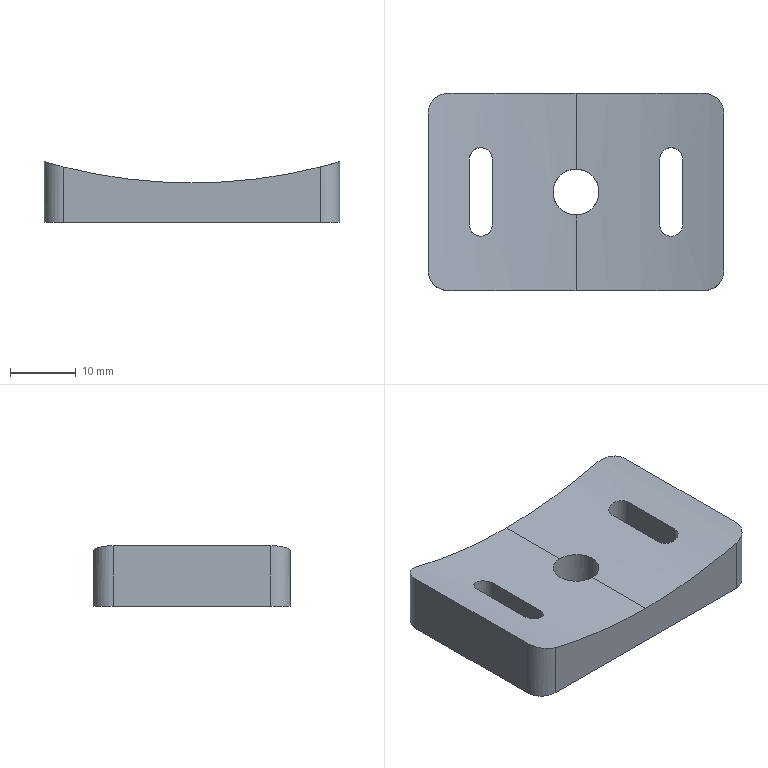Part | SolidWorks | features ICE 2, Extrusion 1, Fillet 1, HoleWzd 1 | 1 solid | 31 faces | box 45 x 30 x 9.229 mm | volume 8297 mm3 | cylinder 16 | plane 15 | commonest cylinder face diameters 6 x8 3.5 x4 7 x2 160 x2
STEP:
#1=CARTESIAN_POINT('',(3.5,15.,-79.923));
#2=VERTEX_POINT('',#1);
#3=CARTESIAN_POINT('',(0.,11.5,-80.));
#4=VERTEX_POINT('',#3);
#5=CARTESIAN_POINT('',(3.5,15.,-79.923));
#6=CARTESIAN_POINT('',(3.5,14.771,-79.923));
#7=CARTESIAN_POINT('',(3.478,14.544,-79.924));
#8=CARTESIAN_POINT('',(3.388,14.093,-79.928));
#9=CARTESIAN_POINT('',(3.321,13.872,-79.931));
#10=CARTESIAN_POINT('',(3.146,13.45,-79.938));
#11=CARTESIAN_POINT('',(3.038,13.247,-79.942));
#12=CARTESIAN_POINT('',(2.782,12.864,-79.952));
#13=CARTESIAN_POINT('',(2.637,12.687,-79.957));
#14=CARTESIAN_POINT('',(2.314,12.364,-79.967));
#15=CARTESIAN_POINT('',(2.134,12.217,-79.972));
#16=CARTESIAN_POINT('',(1.753,11.962,-79.981));
#17=CARTESIAN_POINT('',(1.552,11.855,-79.985));
#18=CARTESIAN_POINT('',(1.129,11.679,-79.992));
#19=CARTESIAN_POINT('',(0.906,11.612,-79.995));
#20=CARTESIAN_POINT('',(0.4583,11.523,-79.999));
#21=CARTESIAN_POINT('',(0.231,11.5,-80.));
#22=CARTESIAN_POINT('',(0.,11.5,-80.));
#23=B_SPLINE_CURVE_WITH_KNOTS('',3,(#5,#6,#7,#8,#9,#10,#11,#12,#13,#14,#15,#16,#17,#18,#19,#20,#21,#22),.UNSPECIFIED.,.F.,.F.,(4,2,2,2,2,2,2,2,4),(0.01094,0.01163,0.01231,0.013,0.01368,0.01436,0.01505,0.01573,0.01642),.UNSPECIFIED.);
#24=EDGE_CURVE('',#2,#4,#23,.T.);
#25=ORIENTED_EDGE('',*,*,#24,.F.);
#26=CARTESIAN_POINT('',(3.5,15.,-86.));
#27=VERTEX_POINT('',#26);
#28=CARTESIAN_POINT('',(3.5,15.,-86.));
#29=DIRECTION('',(0.,0.,-1.));
#30=VECTOR('',#29,1000.);
#31=LINE('',#28,#30);
#32=EDGE_CURVE('',#2,#27,#31,.T.);
#33=ORIENTED_EDGE('',*,*,#32,.T.);
#34=CARTESIAN_POINT('',(-3.5,15.,-86.));
#35=VERTEX_POINT('',#34);
#36=CARTESIAN_POINT('',(0.,15.,-86.));
#37=DIRECTION('',(0.,0.,-1.));
#38=DIRECTION('',(-1.,0.,0.));
#39=AXIS2_PLACEMENT_3D('',#36,#37,#38);
#40=CIRCLE('',#39,3.5);
#41=EDGE_CURVE('',#27,#35,#40,.T.);
#42=ORIENTED_EDGE('',*,*,#41,.T.);
#43=CARTESIAN_POINT('',(-3.5,15.,-79.923));
#44=VERTEX_POINT('',#43);
#45=CARTESIAN_POINT('',(-3.5,15.,-86.));
#46=DIRECTION('',(0.,0.,-1.));
#47=VECTOR('',#46,1000.);
#48=LINE('',#45,#47);
#49=EDGE_CURVE('',#44,#35,#48,.T.);
#50=ORIENTED_EDGE('',*,*,#49,.F.);
#51=CARTESIAN_POINT('',(0.,11.5,-80.));
#52=CARTESIAN_POINT('',(-0.2308,11.5,-80.));
#53=CARTESIAN_POINT('',(-0.4588,11.523,-79.999));
#54=CARTESIAN_POINT('',(-0.9058,11.612,-79.995));
#55=CARTESIAN_POINT('',(-1.128,11.679,-79.992));
#56=CARTESIAN_POINT('',(-1.552,11.854,-79.985));
#57=CARTESIAN_POINT('',(-1.753,11.962,-79.981));
#58=CARTESIAN_POINT('',(-2.133,12.215,-79.972));
#59=CARTESIAN_POINT('',(-2.313,12.363,-79.967));
#60=CARTESIAN_POINT('',(-2.636,12.686,-79.957));
#61=CARTESIAN_POINT('',(-2.78,12.862,-79.952));
#62=CARTESIAN_POINT('',(-3.036,13.243,-79.942));
#63=CARTESIAN_POINT('',(-3.145,13.447,-79.938));
#64=CARTESIAN_POINT('',(-3.407,14.079,-79.928));
#65=CARTESIAN_POINT('',(-3.5,14.538,-79.923));
#66=CARTESIAN_POINT('',(-3.5,15.,-79.923));
#67=B_SPLINE_CURVE_WITH_KNOTS('',3,(#51,#52,#53,#54,#55,#56,#57,#58,#59,#60,#61,#62,#63,#64,#65,#66),.UNSPECIFIED.,.F.,.F.,(4,2,2,2,2,2,2,4),(0.01642,0.0171,0.01778,0.01847,0.01915,0.01983,0.02052,0.02189),.UNSPECIFIED.);
#68=EDGE_CURVE('',#4,#44,#67,.T.);
#69=ORIENTED_EDGE('',*,*,#68,.F.);
#70=EDGE_LOOP('',(#25,#33,#42,#50,#69));
#71=FACE_OUTER_BOUND('',#70,.T.);
#72=CARTESIAN_POINT('',(0.,15.,-86.));
#73=DIRECTION('',(0.,0.,-1.));
#74=DIRECTION('',(-1.,0.,0.));
#75=AXIS2_PLACEMENT_3D('',#72,#73,#74);
#76=CYLINDRICAL_SURFACE('',#75,3.5);
#77=ADVANCED_FACE('',(#71),#76,.F.);
#78=CARTESIAN_POINT('',(12.75,10.,-78.977));
#79=VERTEX_POINT('',#78);
#80=CARTESIAN_POINT('',(12.75,20.,-78.977));
#81=VERTEX_POINT('',#80);
#82=CARTESIAN_POINT('',(12.75,30.,-78.977));
#83=DIRECTION('',(0.,1.,0.));
#84=VECTOR('',#83,1000.);
#85=LINE('',#82,#84);
#86=EDGE_CURVE('',#79,#81,#85,.T.);
#87=ORIENTED_EDGE('',*,*,#86,.T.);
#88=CARTESIAN_POINT('',(16.25,20.,-78.332));
#89=VERTEX_POINT('',#88);
#90=CARTESIAN_POINT('',(12.75,20.,-78.977));
#91=CARTESIAN_POINT('',(12.75,20.117,-78.977));
#92=CARTESIAN_POINT('',(12.762,20.231,-78.976));
#93=CARTESIAN_POINT('',(12.807,20.457,-78.968));
#94=CARTESIAN_POINT('',(12.841,20.569,-78.963));
#95=CARTESIAN_POINT('',(12.93,20.782,-78.948));
#96=CARTESIAN_POINT('',(12.984,20.882,-78.939));
#97=CARTESIAN_POINT('',(13.113,21.073,-78.918));
#98=CARTESIAN_POINT('',(13.187,21.163,-78.906));
#99=CARTESIAN_POINT('',(13.431,21.404,-78.865));
#100=CARTESIAN_POINT('',(13.627,21.533,-78.831));
#101=CARTESIAN_POINT('',(14.047,21.705,-78.757));
#102=CARTESIAN_POINT('',(14.275,21.75,-78.716));
#103=CARTESIAN_POINT('',(14.615,21.75,-78.654));
#104=CARTESIAN_POINT('',(14.73,21.739,-78.632));
#105=CARTESIAN_POINT('',(14.952,21.694,-78.59));
#106=CARTESIAN_POINT('',(15.06,21.662,-78.57));
#107=CARTESIAN_POINT('',(15.271,21.575,-78.529));
#108=CARTESIAN_POINT('',(15.373,21.521,-78.509));
#109=CARTESIAN_POINT('',(15.562,21.396,-78.472));
#110=CARTESIAN_POINT('',(15.65,21.324,-78.454));
#111=CARTESIAN_POINT('',(15.896,21.08,-78.405));
#112=CARTESIAN_POINT('',(16.025,20.888,-78.379));
#113=CARTESIAN_POINT('',(16.204,20.462,-78.342));
#114=CARTESIAN_POINT('',(16.25,20.233,-78.332));
#115=CARTESIAN_POINT('',(16.25,20.,-78.332));
#116=B_SPLINE_CURVE_WITH_KNOTS('',3,(#90,#91,#92,#93,#94,#95,#96,#97,#98,#99,#100,#101,#102,#103,#104,#105,#106,#107,#108,#109,#110,#111,#112,#113,#114,#115),.UNSPECIFIED.,.F.,.F.,(4,2,2,2,2,2,2,2,2,2,2,2,4),(0.,0.0003448,0.0006897,0.001035,0.001379,0.002069,0.002759,0.003104,0.003448,0.003793,0.004138,0.004828,0.005517),.UNSPECIFIED.);
#117=EDGE_CURVE('',#81,#89,#116,.T.);
#118=ORIENTED_EDGE('',*,*,#117,.T.);
#119=CARTESIAN_POINT('',(16.25,10.,-78.332));
#120=VERTEX_POINT('',#119);
#121=CARTESIAN_POINT('',(16.25,30.,-78.332));
#122=DIRECTION('',(0.,-1.,0.));
#123=VECTOR('',#122,1000.);
#124=LINE('',#121,#123);
#125=EDGE_CURVE('',#89,#120,#124,.T.);
#126=ORIENTED_EDGE('',*,*,#125,.T.);
#127=CARTESIAN_POINT('',(16.25,10.,-78.332));
#128=CARTESIAN_POINT('',(16.25,9.77,-78.332));
#129=CARTESIAN_POINT('',(16.203,9.538,-78.342));
#130=CARTESIAN_POINT('',(16.027,9.115,-78.378));
#131=CARTESIAN_POINT('',(15.895,8.919,-78.405));
#132=CARTESIAN_POINT('',(15.653,8.678,-78.454));
#133=CARTESIAN_POINT('',(15.563,8.605,-78.472));
#134=CARTESIAN_POINT('',(15.373,8.479,-78.509));
#135=CARTESIAN_POINT('',(15.273,8.426,-78.529));
#136=CARTESIAN_POINT('',(15.062,8.339,-78.569));
#137=CARTESIAN_POINT('',(14.952,8.306,-78.59));
#138=CARTESIAN_POINT('',(14.731,8.262,-78.632));
#139=CARTESIAN_POINT('',(14.618,8.25,-78.653));
#140=CARTESIAN_POINT('',(14.389,8.25,-78.696));
#141=CARTESIAN_POINT('',(14.276,8.261,-78.716));
#142=CARTESIAN_POINT('',(14.054,8.304,-78.756));
#143=CARTESIAN_POINT('',(13.943,8.337,-78.776));
#144=CARTESIAN_POINT('',(13.732,8.424,-78.813));
#145=CARTESIAN_POINT('',(13.631,8.477,-78.83));
#146=CARTESIAN_POINT('',(13.441,8.602,-78.863));
#147=CARTESIAN_POINT('',(13.35,8.676,-78.878));
#148=CARTESIAN_POINT('',(13.188,8.836,-78.906));
#149=CARTESIAN_POINT('',(13.115,8.924,-78.918));
#150=CARTESIAN_POINT('',(12.986,9.115,-78.939));
#151=CARTESIAN_POINT('',(12.93,9.218,-78.948));
#152=CARTESIAN_POINT('',(12.797,9.535,-78.97));
#153=CARTESIAN_POINT('',(12.75,9.767,-78.977));
#154=CARTESIAN_POINT('',(12.75,10.,-78.977));
#155=B_SPLINE_CURVE_WITH_KNOTS('',3,(#127,#128,#129,#130,#131,#132,#133,#134,#135,#136,#137,#138,#139,#140,#141,#142,#143,#144,#145,#146,#147,#148,#149,#150,#151,#152,#153,#154),.UNSPECIFIED.,.F.,.F.,(4,2,2,2,2,2,2,2,2,2,2,2,2,4),(0.005518,0.006208,0.006898,0.007243,0.007587,0.007932,0.008277,0.008622,0.008967,0.009311,0.009656,0.01,0.01035,0.01104),.UNSPECIFIED.);
#156=EDGE_CURVE('',#120,#79,#155,.T.);
#157=ORIENTED_EDGE('',*,*,#156,.T.);
#158=EDGE_LOOP('',(#87,#118,#126,#157));
#159=FACE_BOUND('',#158,.T.);
#160=CARTESIAN_POINT('',(0.,30.,-80.));
#161=VERTEX_POINT('',#160);
#162=CARTESIAN_POINT('',(19.5,30.,-77.587));
#163=VERTEX_POINT('',#162);
#164=CARTESIAN_POINT('',(0.,30.,0.));
#165=DIRECTION('',(0.,-1.,0.));
#166=DIRECTION('',(0.,0.,1.));
#167=AXIS2_PLACEMENT_3D('',#164,#165,#166);
#168=CIRCLE('',#167,80.);
#169=EDGE_CURVE('',#161,#163,#168,.T.);
#170=ORIENTED_EDGE('',*,*,#169,.F.);
#171=CARTESIAN_POINT('',(0.,18.5,-80.));
#172=VERTEX_POINT('',#171);
#173=CARTESIAN_POINT('',(0.,30.,-80.));
#174=DIRECTION('',(0.,-1.,0.));
#175=VECTOR('',#174,1000.);
#176=LINE('',#173,#175);
#177=EDGE_CURVE('',#161,#172,#176,.T.);
#178=ORIENTED_EDGE('',*,*,#177,.T.);
#179=CARTESIAN_POINT('',(0.,18.5,-80.));
#180=CARTESIAN_POINT('',(0.2283,18.5,-80.));
#181=CARTESIAN_POINT('',(0.4601,18.477,-79.999));
#182=CARTESIAN_POINT('',(0.9089,18.388,-79.995));
#183=CARTESIAN_POINT('',(1.127,18.322,-79.992));
#184=CARTESIAN_POINT('',(1.551,18.146,-79.985));
#185=CARTESIAN_POINT('',(1.756,18.036,-79.981));
#186=CARTESIAN_POINT('',(2.135,17.783,-79.972));
#187=CARTESIAN_POINT('',(2.311,17.638,-79.967));
#188=CARTESIAN_POINT('',(2.638,17.312,-79.957));
#189=CARTESIAN_POINT('',(2.783,17.135,-79.952));
#190=CARTESIAN_POINT('',(3.036,16.756,-79.942));
#191=CARTESIAN_POINT('',(3.146,16.551,-79.938));
#192=CARTESIAN_POINT('',(3.322,16.127,-79.931));
#193=CARTESIAN_POINT('',(3.388,15.909,-79.928));
#194=CARTESIAN_POINT('',(3.477,15.46,-79.924));
#195=CARTESIAN_POINT('',(3.5,15.228,-79.923));
#196=CARTESIAN_POINT('',(3.5,15.,-79.923));
#197=B_SPLINE_CURVE_WITH_KNOTS('',3,(#179,#180,#181,#182,#183,#184,#185,#186,#187,#188,#189,#190,#191,#192,#193,#194,#195,#196),.UNSPECIFIED.,.F.,.F.,(4,2,2,2,2,2,2,2,4),(0.005473,0.006157,0.006841,0.007525,0.008209,0.008892,0.009576,0.01026,0.01094),.UNSPECIFIED.);
#198=EDGE_CURVE('',#172,#2,#197,.T.);
#199=ORIENTED_EDGE('',*,*,#198,.T.);
#200=ORIENTED_EDGE('',*,*,#24,.T.);
#201=CARTESIAN_POINT('',(0.,0.,-80.));
#202=VERTEX_POINT('',#201);
#203=CARTESIAN_POINT('',(0.,30.,-80.));
#204=DIRECTION('',(0.,-1.,0.));
#205=VECTOR('',#204,1000.);
#206=LINE('',#203,#205);
#207=EDGE_CURVE('',#4,#202,#206,.T.);
#208=ORIENTED_EDGE('',*,*,#207,.T.);
#209=CARTESIAN_POINT('',(19.5,0.,-77.587));
#210=VERTEX_POINT('',#209);
#211=CARTESIAN_POINT('',(0.,0.,0.));
#212=DIRECTION('',(0.,-1.,0.));
#213=DIRECTION('',(0.,0.,1.));
#214=AXIS2_PLACEMENT_3D('',#211,#212,#213);
#215=CIRCLE('',#214,80.);
#216=EDGE_CURVE('',#202,#210,#215,.T.);
#217=ORIENTED_EDGE('',*,*,#216,.T.);
#218=CARTESIAN_POINT('',(22.5,3.,-76.771));
#219=VERTEX_POINT('',#218);
#220=CARTESIAN_POINT('',(19.5,0.,-77.587));
#221=CARTESIAN_POINT('',(19.696,0.,-77.538));
#222=CARTESIAN_POINT('',(19.888,0.01893,-77.489));
#223=CARTESIAN_POINT('',(20.266,0.09302,-77.391));
#224=CARTESIAN_POINT('',(20.453,0.1489,-77.341));
#225=CARTESIAN_POINT('',(20.814,0.296,-77.245));
#226=CARTESIAN_POINT('',(20.985,0.386,-77.199));
#227=CARTESIAN_POINT('',(21.309,0.5991,-77.11));
#228=CARTESIAN_POINT('',(21.464,0.7237,-77.067));
#229=CARTESIAN_POINT('',(21.743,0.998,-76.989));
#230=CARTESIAN_POINT('',(21.868,1.148,-76.953));
#231=CARTESIAN_POINT('',(22.09,1.474,-76.89));
#232=CARTESIAN_POINT('',(22.187,1.65,-76.862));
#233=CARTESIAN_POINT('',(22.417,2.197,-76.795));
#234=CARTESIAN_POINT('',(22.5,2.596,-76.771));
#235=CARTESIAN_POINT('',(22.5,3.,-76.771));
#236=B_SPLINE_CURVE_WITH_KNOTS('',3,(#220,#221,#222,#223,#224,#225,#226,#227,#228,#229,#230,#231,#232,#233,#234,#235),.UNSPECIFIED.,.F.,.F.,(4,2,2,2,2,2,2,4),(0.,0.0005963,0.001193,0.001789,0.002385,0.002981,0.003578,0.00477),.UNSPECIFIED.);
#237=EDGE_CURVE('',#210,#219,#236,.T.);
#238=ORIENTED_EDGE('',*,*,#237,.T.);
#239=CARTESIAN_POINT('',(22.5,27.,-76.771));
#240=VERTEX_POINT('',#239);
#241=CARTESIAN_POINT('',(22.5,30.,-76.771));
#242=DIRECTION('',(0.,-1.,0.));
#243=VECTOR('',#242,1000.);
#244=LINE('',#241,#243);
#245=EDGE_CURVE('',#240,#219,#244,.T.);
#246=ORIENTED_EDGE('',*,*,#245,.F.);
#247=CARTESIAN_POINT('',(22.5,27.,-76.771));
#248=CARTESIAN_POINT('',(22.5,27.202,-76.771));
#249=CARTESIAN_POINT('',(22.48,27.4,-76.777));
#250=CARTESIAN_POINT('',(22.401,27.789,-76.8));
#251=CARTESIAN_POINT('',(22.342,27.982,-76.817));
#252=CARTESIAN_POINT('',(22.187,28.348,-76.862));
#253=CARTESIAN_POINT('',(22.093,28.521,-76.889));
#254=CARTESIAN_POINT('',(21.871,28.848,-76.952));
#255=CARTESIAN_POINT('',(21.744,29.001,-76.989));
#256=CARTESIAN_POINT('',(21.327,29.412,-77.105));
#257=CARTESIAN_POINT('',(20.993,29.63,-77.197));
#258=CARTESIAN_POINT('',(20.457,29.85,-77.34));
#259=CARTESIAN_POINT('',(20.269,29.906,-77.39));
#260=CARTESIAN_POINT('',(19.888,29.981,-77.489));
#261=CARTESIAN_POINT('',(19.695,30.,-77.538));
#262=CARTESIAN_POINT('',(19.5,30.,-77.587));
#263=B_SPLINE_CURVE_WITH_KNOTS('',3,(#247,#248,#249,#250,#251,#252,#253,#254,#255,#256,#257,#258,#259,#260,#261,#262),.UNSPECIFIED.,.F.,.F.,(4,2,2,2,2,2,2,4),(0.,0.0005963,0.001193,0.001789,0.002385,0.003578,0.004174,0.00477),.UNSPECIFIED.);
#264=EDGE_CURVE('',#240,#163,#263,.T.);
#265=ORIENTED_EDGE('',*,*,#264,.T.);
#266=EDGE_LOOP('',(#170,#178,#199,#200,#208,#217,#238,#246,#265));
#267=FACE_OUTER_BOUND('',#266,.T.);
#268=CARTESIAN_POINT('',(0.,30.,0.));
#269=DIRECTION('',(0.,-1.,0.));
#270=DIRECTION('',(0.,0.,-1.));
#271=AXIS2_PLACEMENT_3D('',#268,#269,#270);
#272=CYLINDRICAL_SURFACE('',#271,80.);
#273=ADVANCED_FACE('',(#159,#267),#272,.F.);
#274=CARTESIAN_POINT('',(-12.75,20.,-82.7));
#275=VERTEX_POINT('',#274);
#276=CARTESIAN_POINT('',(-16.25,20.,-82.7));
#277=VERTEX_POINT('',#276);
#278=CARTESIAN_POINT('',(-14.5,20.,-82.7));
#279=DIRECTION('',(0.,0.,1.));
#280=DIRECTION('',(-1.,0.,0.));
#281=AXIS2_PLACEMENT_3D('',#278,#279,#280);
#282=CIRCLE('',#281,1.75);
#283=EDGE_CURVE('',#275,#277,#282,.T.);
#284=ORIENTED_EDGE('',*,*,#283,.F.);
#285=CARTESIAN_POINT('',(-12.75,20.,-78.977));
#286=VERTEX_POINT('',#285);
#287=CARTESIAN_POINT('',(-12.75,20.,-76.586));
#288=DIRECTION('',(0.,0.,-1.));
#289=VECTOR('',#288,1000.);
#290=LINE('',#287,#289);
#291=EDGE_CURVE('',#286,#275,#290,.T.);
#292=ORIENTED_EDGE('',*,*,#291,.F.);
#293=CARTESIAN_POINT('',(-16.25,20.,-78.332));
#294=VERTEX_POINT('',#293);
#295=CARTESIAN_POINT('',(-16.25,20.,-78.332));
#296=CARTESIAN_POINT('',(-16.25,20.117,-78.332));
#297=CARTESIAN_POINT('',(-16.238,20.231,-78.335));
#298=CARTESIAN_POINT('',(-16.193,20.457,-78.344));
#299=CARTESIAN_POINT('',(-16.159,20.568,-78.351));
#300=CARTESIAN_POINT('',(-16.07,20.781,-78.369));
#301=CARTESIAN_POINT('',(-16.016,20.882,-78.38));
#302=CARTESIAN_POINT('',(-15.888,21.072,-78.407));
#303=CARTESIAN_POINT('',(-15.814,21.162,-78.422));
#304=CARTESIAN_POINT('',(-15.571,21.403,-78.47));
#305=CARTESIAN_POINT('',(-15.376,21.532,-78.509));
#306=CARTESIAN_POINT('',(-14.958,21.704,-78.59));
#307=CARTESIAN_POINT('',(-14.73,21.75,-78.633));
#308=CARTESIAN_POINT('',(-14.39,21.75,-78.695));
#309=CARTESIAN_POINT('',(-14.275,21.739,-78.716));
#310=CARTESIAN_POINT('',(-14.052,21.696,-78.756));
#311=CARTESIAN_POINT('',(-13.944,21.663,-78.776));
#312=CARTESIAN_POINT('',(-13.732,21.577,-78.813));
#313=CARTESIAN_POINT('',(-13.63,21.523,-78.83));
#314=CARTESIAN_POINT('',(-13.44,21.397,-78.863));
#315=CARTESIAN_POINT('',(-13.351,21.325,-78.878));
#316=CARTESIAN_POINT('',(-13.105,21.081,-78.92));
#317=CARTESIAN_POINT('',(-12.975,20.889,-78.941));
#318=CARTESIAN_POINT('',(-12.796,20.462,-78.97));
#319=CARTESIAN_POINT('',(-12.75,20.233,-78.977));
#320=CARTESIAN_POINT('',(-12.75,20.,-78.977));
#321=B_SPLINE_CURVE_WITH_KNOTS('',3,(#295,#296,#297,#298,#299,#300,#301,#302,#303,#304,#305,#306,#307,#308,#309,#310,#311,#312,#313,#314,#315,#316,#317,#318,#319,#320),.UNSPECIFIED.,.F.,.F.,(4,2,2,2,2,2,2,2,2,2,2,2,4),(0.,0.0003448,0.0006897,0.001034,0.001379,0.002069,0.002759,0.003103,0.003448,0.003793,0.004138,0.004828,0.005517),.UNSPECIFIED.);
#322=EDGE_CURVE('',#294,#286,#321,.T.);
#323=ORIENTED_EDGE('',*,*,#322,.F.);
#324=CARTESIAN_POINT('',(-16.25,20.,-76.586));
#325=DIRECTION('',(0.,0.,-1.));
#326=VECTOR('',#325,1000.);
#327=LINE('',#324,#326);
#328=EDGE_CURVE('',#294,#277,#327,.T.);
#329=ORIENTED_EDGE('',*,*,#328,.T.);
#330=EDGE_LOOP('',(#284,#292,#323,#329));
#331=FACE_OUTER_BOUND('',#330,.T.);
#332=CARTESIAN_POINT('',(-14.5,20.,-76.586));
#333=DIRECTION('',(0.,0.,-1.));
#334=DIRECTION('',(-1.,0.,0.));
#335=AXIS2_PLACEMENT_3D('',#332,#333,#334);
#336=CYLINDRICAL_SURFACE('',#335,1.75);
#337=ADVANCED_FACE('',(#331),#336,.F.);
#338=CARTESIAN_POINT('',(-16.25,10.,-82.7));
#339=VERTEX_POINT('',#338);
#340=CARTESIAN_POINT('',(-16.25,20.,-82.7));
#341=DIRECTION('',(0.,-1.,0.));
#342=VECTOR('',#341,1000.);
#343=LINE('',#340,#342);
#344=EDGE_CURVE('',#277,#339,#343,.T.);
#345=ORIENTED_EDGE('',*,*,#344,.F.);
#346=ORIENTED_EDGE('',*,*,#328,.F.);
#347=CARTESIAN_POINT('',(-16.25,10.,-78.332));
#348=VERTEX_POINT('',#347);
#349=CARTESIAN_POINT('',(-16.25,30.,-78.332));
#350=DIRECTION('',(0.,1.,0.));
#351=VECTOR('',#350,1000.);
#352=LINE('',#349,#351);
#353=EDGE_CURVE('',#348,#294,#352,.T.);
#354=ORIENTED_EDGE('',*,*,#353,.F.);
#355=CARTESIAN_POINT('',(-16.25,10.,-76.586));
#356=DIRECTION('',(0.,0.,-1.));
#357=VECTOR('',#356,1000.);
#358=LINE('',#355,#357);
#359=EDGE_CURVE('',#348,#339,#358,.T.);
#360=ORIENTED_EDGE('',*,*,#359,.T.);
#361=EDGE_LOOP('',(#345,#346,#354,#360));
#362=FACE_OUTER_BOUND('',#361,.T.);
#363=CARTESIAN_POINT('',(-16.25,20.,-76.586));
#364=DIRECTION('',(-1.,0.,0.));
#365=DIRECTION('',(0.,0.,1.));
#366=AXIS2_PLACEMENT_3D('',#363,#364,#365);
#367=PLANE('',#366);
#368=ADVANCED_FACE('',(#362),#367,.F.);
#369=CARTESIAN_POINT('',(-12.75,10.,-82.7));
#370=VERTEX_POINT('',#369);
#371=CARTESIAN_POINT('',(-14.5,10.,-82.7));
#372=DIRECTION('',(0.,0.,1.));
#373=DIRECTION('',(-1.,0.,0.));
#374=AXIS2_PLACEMENT_3D('',#371,#372,#373);
#375=CIRCLE('',#374,1.75);
#376=EDGE_CURVE('',#339,#370,#375,.T.);
#377=ORIENTED_EDGE('',*,*,#376,.F.);
#378=ORIENTED_EDGE('',*,*,#359,.F.);
#379=CARTESIAN_POINT('',(-12.75,10.,-78.977));
#380=VERTEX_POINT('',#379);
#381=CARTESIAN_POINT('',(-12.75,10.,-78.977));
#382=CARTESIAN_POINT('',(-12.75,9.77,-78.977));
#383=CARTESIAN_POINT('',(-12.797,9.538,-78.97));
#384=CARTESIAN_POINT('',(-12.973,9.114,-78.941));
#385=CARTESIAN_POINT('',(-13.105,8.919,-78.919));
#386=CARTESIAN_POINT('',(-13.349,8.677,-78.878));
#387=CARTESIAN_POINT('',(-13.439,8.603,-78.863));
#388=CARTESIAN_POINT('',(-13.63,8.478,-78.83));
#389=CARTESIAN_POINT('',(-13.73,8.424,-78.813));
#390=CARTESIAN_POINT('',(-13.942,8.338,-78.776));
#391=CARTESIAN_POINT('',(-14.052,8.305,-78.756));
#392=CARTESIAN_POINT('',(-14.274,8.261,-78.716));
#393=CARTESIAN_POINT('',(-14.387,8.25,-78.696));
#394=CARTESIAN_POINT('',(-14.616,8.25,-78.654));
#395=CARTESIAN_POINT('',(-14.729,8.261,-78.633));
#396=CARTESIAN_POINT('',(-14.951,8.305,-78.591));
#397=CARTESIAN_POINT('',(-15.061,8.338,-78.57));
#398=CARTESIAN_POINT('',(-15.272,8.425,-78.529));
#399=CARTESIAN_POINT('',(-15.372,8.478,-78.509));
#400=CARTESIAN_POINT('',(-15.561,8.604,-78.472));
#401=CARTESIAN_POINT('',(-15.651,8.677,-78.454));
#402=CARTESIAN_POINT('',(-15.813,8.838,-78.422));
#403=CARTESIAN_POINT('',(-15.886,8.925,-78.407));
#404=CARTESIAN_POINT('',(-16.015,9.116,-78.381));
#405=CARTESIAN_POINT('',(-16.07,9.218,-78.369));
#406=CARTESIAN_POINT('',(-16.203,9.535,-78.342));
#407=CARTESIAN_POINT('',(-16.25,9.767,-78.332));
#408=CARTESIAN_POINT('',(-16.25,10.,-78.332));
#409=B_SPLINE_CURVE_WITH_KNOTS('',3,(#381,#382,#383,#384,#385,#386,#387,#388,#389,#390,#391,#392,#393,#394,#395,#396,#397,#398,#399,#400,#401,#402,#403,#404,#405,#406,#407,#408),.UNSPECIFIED.,.F.,.F.,(4,2,2,2,2,2,2,2,2,2,2,2,2,4),(0.005518,0.006208,0.006898,0.007243,0.007587,0.007932,0.008277,0.008622,0.008967,0.009311,0.009656,0.01,0.01035,0.01104),.UNSPECIFIED.);
#410=EDGE_CURVE('',#380,#348,#409,.T.);
#411=ORIENTED_EDGE('',*,*,#410,.F.);
#412=CARTESIAN_POINT('',(-12.75,10.,-76.586));
#413=DIRECTION('',(0.,0.,-1.));
#414=VECTOR('',#413,1000.);
#415=LINE('',#412,#414);
#416=EDGE_CURVE('',#380,#370,#415,.T.);
#417=ORIENTED_EDGE('',*,*,#416,.T.);
#418=EDGE_LOOP('',(#377,#378,#411,#417));
#419=FACE_OUTER_BOUND('',#418,.T.);
#420=CARTESIAN_POINT('',(-14.5,10.,-76.586));
#421=DIRECTION('',(0.,0.,-1.));
#422=DIRECTION('',(-1.,0.,0.));
#423=AXIS2_PLACEMENT_3D('',#420,#421,#422);
#424=CYLINDRICAL_SURFACE('',#423,1.75);
#425=ADVANCED_FACE('',(#419),#424,.F.);
#426=CARTESIAN_POINT('',(-12.75,20.,-82.7));
#427=DIRECTION('',(0.,1.,0.));
#428=VECTOR('',#427,1000.);
#429=LINE('',#426,#428);
#430=EDGE_CURVE('',#370,#275,#429,.T.);
#431=ORIENTED_EDGE('',*,*,#430,.F.);
#432=ORIENTED_EDGE('',*,*,#416,.F.);
#433=CARTESIAN_POINT('',(-12.75,30.,-78.977));
#434=DIRECTION('',(0.,-1.,0.));
#435=VECTOR('',#434,1000.);
#436=LINE('',#433,#435);
#437=EDGE_CURVE('',#286,#380,#436,.T.);
#438=ORIENTED_EDGE('',*,*,#437,.F.);
#439=ORIENTED_EDGE('',*,*,#291,.T.);
#440=EDGE_LOOP('',(#431,#432,#438,#439));
#441=FACE_OUTER_BOUND('',#440,.T.);
#442=CARTESIAN_POINT('',(-12.75,20.,-76.586));
#443=DIRECTION('',(1.,0.,0.));
#444=DIRECTION('',(0.,0.,-1.));
#445=AXIS2_PLACEMENT_3D('',#442,#443,#444);
#446=PLANE('',#445);
#447=ADVANCED_FACE('',(#441),#446,.F.);
#448=CARTESIAN_POINT('',(16.25,20.,-82.7));
#449=VERTEX_POINT('',#448);
#450=CARTESIAN_POINT('',(12.75,20.,-82.7));
#451=VERTEX_POINT('',#450);
#452=CARTESIAN_POINT('',(14.5,20.,-82.7));
#453=DIRECTION('',(0.,0.,1.));
#454=DIRECTION('',(-1.,0.,0.));
#455=AXIS2_PLACEMENT_3D('',#452,#453,#454);
#456=CIRCLE('',#455,1.75);
#457=EDGE_CURVE('',#449,#451,#456,.T.);
#458=ORIENTED_EDGE('',*,*,#457,.F.);
#459=CARTESIAN_POINT('',(16.25,20.,-76.586));
#460=DIRECTION('',(0.,0.,-1.));
#461=VECTOR('',#460,1000.);
#462=LINE('',#459,#461);
#463=EDGE_CURVE('',#89,#449,#462,.T.);
#464=ORIENTED_EDGE('',*,*,#463,.F.);
#465=ORIENTED_EDGE('',*,*,#117,.F.);
#466=CARTESIAN_POINT('',(12.75,20.,-76.586));
#467=DIRECTION('',(0.,0.,-1.));
#468=VECTOR('',#467,1000.);
#469=LINE('',#466,#468);
#470=EDGE_CURVE('',#81,#451,#469,.T.);
#471=ORIENTED_EDGE('',*,*,#470,.T.);
#472=EDGE_LOOP('',(#458,#464,#465,#471));
#473=FACE_OUTER_BOUND('',#472,.T.);
#474=CARTESIAN_POINT('',(14.5,20.,-76.586));
#475=DIRECTION('',(0.,0.,-1.));
#476=DIRECTION('',(-1.,0.,0.));
#477=AXIS2_PLACEMENT_3D('',#474,#475,#476);
#478=CYLINDRICAL_SURFACE('',#477,1.75);
#479=ADVANCED_FACE('',(#473),#478,.F.);
#480=CARTESIAN_POINT('',(12.75,10.,-82.7));
#481=VERTEX_POINT('',#480);
#482=CARTESIAN_POINT('',(12.75,20.,-82.7));
#483=DIRECTION('',(0.,-1.,0.));
#484=VECTOR('',#483,1000.);
#485=LINE('',#482,#484);
#486=EDGE_CURVE('',#451,#481,#485,.T.);
#487=ORIENTED_EDGE('',*,*,#486,.F.);
#488=ORIENTED_EDGE('',*,*,#470,.F.);
#489=ORIENTED_EDGE('',*,*,#86,.F.);
#490=CARTESIAN_POINT('',(12.75,10.,-76.586));
#491=DIRECTION('',(0.,0.,-1.));
#492=VECTOR('',#491,1000.);
#493=LINE('',#490,#492);
#494=EDGE_CURVE('',#79,#481,#493,.T.);
#495=ORIENTED_EDGE('',*,*,#494,.T.);
#496=EDGE_LOOP('',(#487,#488,#489,#495));
#497=FACE_OUTER_BOUND('',#496,.T.);
#498=CARTESIAN_POINT('',(12.75,20.,-76.586));
#499=DIRECTION('',(-1.,0.,0.));
#500=DIRECTION('',(0.,-1.,0.));
#501=AXIS2_PLACEMENT_3D('',#498,#499,#500);
#502=PLANE('',#501);
#503=ADVANCED_FACE('',(#497),#502,.F.);
#504=CARTESIAN_POINT('',(16.25,10.,-82.7));
#505=VERTEX_POINT('',#504);
#506=CARTESIAN_POINT('',(14.5,10.,-82.7));
#507=DIRECTION('',(0.,0.,1.));
#508=DIRECTION('',(-1.,0.,0.));
#509=AXIS2_PLACEMENT_3D('',#506,#507,#508);
#510=CIRCLE('',#509,1.75);
#511=EDGE_CURVE('',#481,#505,#510,.T.);
#512=ORIENTED_EDGE('',*,*,#511,.F.);
#513=ORIENTED_EDGE('',*,*,#494,.F.);
#514=ORIENTED_EDGE('',*,*,#156,.F.);
#515=CARTESIAN_POINT('',(16.25,10.,-76.586));
#516=DIRECTION('',(0.,0.,-1.));
#517=VECTOR('',#516,1000.);
#518=LINE('',#515,#517);
#519=EDGE_CURVE('',#120,#505,#518,.T.);
#520=ORIENTED_EDGE('',*,*,#519,.T.);
#521=EDGE_LOOP('',(#512,#513,#514,#520));
#522=FACE_OUTER_BOUND('',#521,.T.);
#523=CARTESIAN_POINT('',(14.5,10.,-76.586));
#524=DIRECTION('',(0.,0.,-1.));
#525=DIRECTION('',(-1.,0.,0.));
#526=AXIS2_PLACEMENT_3D('',#523,#524,#525);
#527=CYLINDRICAL_SURFACE('',#526,1.75);
#528=ADVANCED_FACE('',(#522),#527,.F.);
#529=CARTESIAN_POINT('',(16.25,20.,-82.7));
#530=DIRECTION('',(0.,1.,0.));
#531=VECTOR('',#530,1000.);
#532=LINE('',#529,#531);
#533=EDGE_CURVE('',#505,#449,#532,.T.);
#534=ORIENTED_EDGE('',*,*,#533,.F.);
#535=ORIENTED_EDGE('',*,*,#519,.F.);
#536=ORIENTED_EDGE('',*,*,#125,.F.);
#537=ORIENTED_EDGE('',*,*,#463,.T.);
#538=EDGE_LOOP('',(#534,#535,#536,#537));
#539=FACE_OUTER_BOUND('',#538,.T.);
#540=CARTESIAN_POINT('',(16.25,20.,-76.586));
#541=DIRECTION('',(1.,0.,0.));
#542=DIRECTION('',(0.,1.,0.));
#543=AXIS2_PLACEMENT_3D('',#540,#541,#542);
#544=PLANE('',#543);
#545=ADVANCED_FACE('',(#539),#544,.F.);
#546=CARTESIAN_POINT('',(-11.5,20.,-86.));
#547=VERTEX_POINT('',#546);
#548=CARTESIAN_POINT('',(-11.5,10.,-86.));
#549=VERTEX_POINT('',#548);
#550=CARTESIAN_POINT('',(-11.5,20.,-86.));
#551=DIRECTION('',(0.,-1.,0.));
#552=VECTOR('',#551,1000.);
#553=LINE('',#550,#552);
#554=EDGE_CURVE('',#547,#549,#553,.T.);
#555=ORIENTED_EDGE('',*,*,#554,.F.);
#556=CARTESIAN_POINT('',(-17.5,20.,-86.));
#557=VERTEX_POINT('',#556);
#558=CARTESIAN_POINT('',(-14.5,20.,-86.));
#559=DIRECTION('',(0.,0.,-1.));
#560=DIRECTION('',(-1.,0.,0.));
#561=AXIS2_PLACEMENT_3D('',#558,#559,#560);
#562=CIRCLE('',#561,3.);
#563=EDGE_CURVE('',#557,#547,#562,.T.);
#564=ORIENTED_EDGE('',*,*,#563,.F.);
#565=CARTESIAN_POINT('',(-17.5,10.,-86.));
#566=VERTEX_POINT('',#565);
#567=CARTESIAN_POINT('',(-17.5,20.,-86.));
#568=DIRECTION('',(0.,1.,0.));
#569=VECTOR('',#568,1000.);
#570=LINE('',#567,#569);
#571=EDGE_CURVE('',#566,#557,#570,.T.);
#572=ORIENTED_EDGE('',*,*,#571,.F.);
#573=CARTESIAN_POINT('',(-14.5,10.,-86.));
#574=DIRECTION('',(0.,0.,-1.));
#575=DIRECTION('',(-1.,0.,0.));
#576=AXIS2_PLACEMENT_3D('',#573,#574,#575);
#577=CIRCLE('',#576,3.);
#578=EDGE_CURVE('',#549,#566,#577,.T.);
#579=ORIENTED_EDGE('',*,*,#578,.F.);
#580=EDGE_LOOP('',(#555,#564,#572,#579));
#581=FACE_BOUND('',#580,.T.);
#582=CARTESIAN_POINT('',(17.5,20.,-86.));
#583=VERTEX_POINT('',#582);
#584=CARTESIAN_POINT('',(17.5,10.,-86.));
#585=VERTEX_POINT('',#584);
#586=CARTESIAN_POINT('',(17.5,20.,-86.));
#587=DIRECTION('',(0.,-1.,0.));
#588=VECTOR('',#587,1000.);
#589=LINE('',#586,#588);
#590=EDGE_CURVE('',#583,#585,#589,.T.);
#591=ORIENTED_EDGE('',*,*,#590,.F.);
#592=CARTESIAN_POINT('',(11.5,20.,-86.));
#593=VERTEX_POINT('',#592);
#594=CARTESIAN_POINT('',(14.5,20.,-86.));
#595=DIRECTION('',(0.,0.,-1.));
#596=DIRECTION('',(-1.,0.,0.));
#597=AXIS2_PLACEMENT_3D('',#594,#595,#596);
#598=CIRCLE('',#597,3.);
#599=EDGE_CURVE('',#593,#583,#598,.T.);
#600=ORIENTED_EDGE('',*,*,#599,.F.);
#601=CARTESIAN_POINT('',(11.5,10.,-86.));
#602=VERTEX_POINT('',#601);
#603=CARTESIAN_POINT('',(11.5,20.,-86.));
#604=DIRECTION('',(0.,1.,0.));
#605=VECTOR('',#604,1000.);
#606=LINE('',#603,#605);
#607=EDGE_CURVE('',#602,#593,#606,.T.);
#608=ORIENTED_EDGE('',*,*,#607,.F.);
#609=CARTESIAN_POINT('',(14.5,10.,-86.));
#610=DIRECTION('',(0.,0.,-1.));
#611=DIRECTION('',(-1.,0.,0.));
#612=AXIS2_PLACEMENT_3D('',#609,#610,#611);
#613=CIRCLE('',#612,3.);
#614=EDGE_CURVE('',#585,#602,#613,.T.);
#615=ORIENTED_EDGE('',*,*,#614,.F.);
#616=EDGE_LOOP('',(#591,#600,#608,#615));
#617=FACE_BOUND('',#616,.T.);
#618=CARTESIAN_POINT('',(0.,15.,-86.));
#619=DIRECTION('',(0.,0.,-1.));
#620=DIRECTION('',(-1.,0.,0.));
#621=AXIS2_PLACEMENT_3D('',#618,#619,#620);
#622=CIRCLE('',#621,3.5);
#623=EDGE_CURVE('',#35,#27,#622,.T.);
#624=ORIENTED_EDGE('',*,*,#623,.F.);
#625=ORIENTED_EDGE('',*,*,#41,.F.);
#626=EDGE_LOOP('',(#624,#625));
#627=FACE_BOUND('',#626,.T.);
#628=CARTESIAN_POINT('',(19.5,0.,-86.));
#629=VERTEX_POINT('',#628);
#630=CARTESIAN_POINT('',(-19.5,0.,-86.));
#631=VERTEX_POINT('',#630);
#632=CARTESIAN_POINT('',(-22.5,0.,-86.));
#633=DIRECTION('',(-1.,0.,0.));
#634=VECTOR('',#633,1000.);
#635=LINE('',#632,#634);
#636=EDGE_CURVE('',#629,#631,#635,.T.);
#637=ORIENTED_EDGE('',*,*,#636,.T.);
#638=CARTESIAN_POINT('',(-22.5,3.,-86.));
#639=VERTEX_POINT('',#638);
#640=CARTESIAN_POINT('',(-19.5,3.,-86.));
#641=DIRECTION('',(0.,0.,-1.));
#642=DIRECTION('',(1.,0.,0.));
#643=AXIS2_PLACEMENT_3D('',#640,#641,#642);
#644=CIRCLE('',#643,3.);
#645=EDGE_CURVE('',#631,#639,#644,.T.);
#646=ORIENTED_EDGE('',*,*,#645,.T.);
#647=CARTESIAN_POINT('',(-22.5,27.,-86.));
#648=VERTEX_POINT('',#647);
#649=CARTESIAN_POINT('',(-22.5,30.,-86.));
#650=DIRECTION('',(0.,-1.,0.));
#651=VECTOR('',#650,1000.);
#652=LINE('',#649,#651);
#653=EDGE_CURVE('',#648,#639,#652,.T.);
#654=ORIENTED_EDGE('',*,*,#653,.F.);
#655=CARTESIAN_POINT('',(-19.5,30.,-86.));
#656=VERTEX_POINT('',#655);
#657=CARTESIAN_POINT('',(-19.5,27.,-86.));
#658=DIRECTION('',(0.,0.,-1.));
#659=DIRECTION('',(1.,0.,0.));
#660=AXIS2_PLACEMENT_3D('',#657,#658,#659);
#661=CIRCLE('',#660,3.);
#662=EDGE_CURVE('',#648,#656,#661,.T.);
#663=ORIENTED_EDGE('',*,*,#662,.T.);
#664=CARTESIAN_POINT('',(19.5,30.,-86.));
#665=VERTEX_POINT('',#664);
#666=CARTESIAN_POINT('',(-22.5,30.,-86.));
#667=DIRECTION('',(-1.,0.,0.));
#668=VECTOR('',#667,1000.);
#669=LINE('',#666,#668);
#670=EDGE_CURVE('',#665,#656,#669,.T.);
#671=ORIENTED_EDGE('',*,*,#670,.F.);
#672=CARTESIAN_POINT('',(22.5,27.,-86.));
#673=VERTEX_POINT('',#672);
#674=CARTESIAN_POINT('',(19.5,27.,-86.));
#675=DIRECTION('',(0.,0.,-1.));
#676=DIRECTION('',(1.,0.,0.));
#677=AXIS2_PLACEMENT_3D('',#674,#675,#676);
#678=CIRCLE('',#677,3.);
#679=EDGE_CURVE('',#665,#673,#678,.T.);
#680=ORIENTED_EDGE('',*,*,#679,.T.);
#681=CARTESIAN_POINT('',(22.5,3.,-86.));
#682=VERTEX_POINT('',#681);
#683=CARTESIAN_POINT('',(22.5,30.,-86.));
#684=DIRECTION('',(0.,-1.,0.));
#685=VECTOR('',#684,1000.);
#686=LINE('',#683,#685);
#687=EDGE_CURVE('',#673,#682,#686,.T.);
#688=ORIENTED_EDGE('',*,*,#687,.T.);
#689=CARTESIAN_POINT('',(19.5,3.,-86.));
#690=DIRECTION('',(0.,0.,-1.));
#691=DIRECTION('',(1.,0.,0.));
#692=AXIS2_PLACEMENT_3D('',#689,#690,#691);
#693=CIRCLE('',#692,3.);
#694=EDGE_CURVE('',#682,#629,#693,.T.);
#695=ORIENTED_EDGE('',*,*,#694,.T.);
#696=EDGE_LOOP('',(#637,#646,#654,#663,#671,#680,#688,#695));
#697=FACE_OUTER_BOUND('',#696,.T.);
#698=CARTESIAN_POINT('',(-22.5,30.,-86.));
#699=DIRECTION('',(0.,0.,1.));
#700=DIRECTION('',(1.,0.,0.));
#701=AXIS2_PLACEMENT_3D('',#698,#699,#700);
#702=PLANE('',#701);
#703=ADVANCED_FACE('',(#581,#617,#627,#697),#702,.F.);
#704=ORIENTED_EDGE('',*,*,#653,.T.);
#705=CARTESIAN_POINT('',(-22.5,3.,-76.771));
#706=VERTEX_POINT('',#705);
#707=CARTESIAN_POINT('',(-22.5,3.,-76.771));
#708=DIRECTION('',(0.,0.,1.));
#709=VECTOR('',#708,1000.);
#710=LINE('',#707,#709);
#711=EDGE_CURVE('',#639,#706,#710,.T.);
#712=ORIENTED_EDGE('',*,*,#711,.T.);
#713=CARTESIAN_POINT('',(-22.5,27.,-76.771));
#714=VERTEX_POINT('',#713);
#715=CARTESIAN_POINT('',(-22.5,30.,-76.771));
#716=DIRECTION('',(0.,-1.,0.));
#717=VECTOR('',#716,1000.);
#718=LINE('',#715,#717);
#719=EDGE_CURVE('',#714,#706,#718,.T.);
#720=ORIENTED_EDGE('',*,*,#719,.F.);
#721=CARTESIAN_POINT('',(-22.5,27.,-86.));
#722=DIRECTION('',(0.,0.,-1.));
#723=VECTOR('',#722,1000.);
#724=LINE('',#721,#723);
#725=EDGE_CURVE('',#714,#648,#724,.T.);
#726=ORIENTED_EDGE('',*,*,#725,.T.);
#727=EDGE_LOOP('',(#704,#712,#720,#726));
#728=FACE_OUTER_BOUND('',#727,.T.);
#729=CARTESIAN_POINT('',(-22.5,30.,-76.771));
#730=DIRECTION('',(1.,0.,0.));
#731=DIRECTION('',(0.,0.,-1.));
#732=AXIS2_PLACEMENT_3D('',#729,#730,#731);
#733=PLANE('',#732);
#734=ADVANCED_FACE('',(#728),#733,.F.);
#735=ORIENTED_EDGE('',*,*,#177,.F.);
#736=CARTESIAN_POINT('',(-19.5,30.,-77.587));
#737=VERTEX_POINT('',#736);
#738=CARTESIAN_POINT('',(0.,30.,0.));
#739=DIRECTION('',(0.,-1.,0.));
#740=DIRECTION('',(0.,0.,1.));
#741=AXIS2_PLACEMENT_3D('',#738,#739,#740);
#742=CIRCLE('',#741,80.);
#743=EDGE_CURVE('',#737,#161,#742,.T.);
#744=ORIENTED_EDGE('',*,*,#743,.F.);
#745=CARTESIAN_POINT('',(-19.5,30.,-77.587));
#746=CARTESIAN_POINT('',(-19.696,30.,-77.538));
#747=CARTESIAN_POINT('',(-19.888,29.981,-77.489));
#748=CARTESIAN_POINT('',(-20.266,29.907,-77.391));
#749=CARTESIAN_POINT('',(-20.453,29.851,-77.341));
#750=CARTESIAN_POINT('',(-20.814,29.704,-77.245));
#751=CARTESIAN_POINT('',(-20.985,29.614,-77.199));
#752=CARTESIAN_POINT('',(-21.309,29.401,-77.11));
#753=CARTESIAN_POINT('',(-21.464,29.276,-77.067));
#754=CARTESIAN_POINT('',(-21.743,29.002,-76.989));
#755=CARTESIAN_POINT('',(-21.868,28.852,-76.953));
#756=CARTESIAN_POINT('',(-22.09,28.526,-76.89));
#757=CARTESIAN_POINT('',(-22.187,28.35,-76.862));
#758=CARTESIAN_POINT('',(-22.417,27.803,-76.795));
#759=CARTESIAN_POINT('',(-22.5,27.404,-76.771));
#760=CARTESIAN_POINT('',(-22.5,27.,-76.771));
#761=B_SPLINE_CURVE_WITH_KNOTS('',3,(#745,#746,#747,#748,#749,#750,#751,#752,#753,#754,#755,#756,#757,#758,#759,#760),.UNSPECIFIED.,.F.,.F.,(4,2,2,2,2,2,2,4),(0.,0.0005963,0.001193,0.001789,0.002385,0.002981,0.003578,0.00477),.UNSPECIFIED.);
#762=EDGE_CURVE('',#737,#714,#761,.T.);
#763=ORIENTED_EDGE('',*,*,#762,.T.);
#764=ORIENTED_EDGE('',*,*,#719,.T.);
#765=CARTESIAN_POINT('',(-19.5,0.,-77.587));
#766=VERTEX_POINT('',#765);
#767=CARTESIAN_POINT('',(-22.5,3.,-76.771));
#768=CARTESIAN_POINT('',(-22.5,2.798,-76.771));
#769=CARTESIAN_POINT('',(-22.48,2.6,-76.777));
#770=CARTESIAN_POINT('',(-22.401,2.211,-76.8));
#771=CARTESIAN_POINT('',(-22.342,2.018,-76.817));
#772=CARTESIAN_POINT('',(-22.187,1.652,-76.862));
#773=CARTESIAN_POINT('',(-22.093,1.479,-76.889));
#774=CARTESIAN_POINT('',(-21.871,1.152,-76.952));
#775=CARTESIAN_POINT('',(-21.744,0.9991,-76.989));
#776=CARTESIAN_POINT('',(-21.327,0.5885,-77.105));
#777=CARTESIAN_POINT('',(-20.993,0.3696,-77.197));
#778=CARTESIAN_POINT('',(-20.457,0.1503,-77.34));
#779=CARTESIAN_POINT('',(-20.269,0.09384,-77.39));
#780=CARTESIAN_POINT('',(-19.888,0.01891,-77.489));
#781=CARTESIAN_POINT('',(-19.695,0.,-77.538));
#782=CARTESIAN_POINT('',(-19.5,0.,-77.587));
#783=B_SPLINE_CURVE_WITH_KNOTS('',3,(#767,#768,#769,#770,#771,#772,#773,#774,#775,#776,#777,#778,#779,#780,#781,#782),.UNSPECIFIED.,.F.,.F.,(4,2,2,2,2,2,2,4),(0.,0.0005963,0.001193,0.001789,0.002385,0.003578,0.004174,0.00477),.UNSPECIFIED.);
#784=EDGE_CURVE('',#706,#766,#783,.T.);
#785=ORIENTED_EDGE('',*,*,#784,.T.);
#786=CARTESIAN_POINT('',(0.,0.,0.));
#787=DIRECTION('',(0.,-1.,0.));
#788=DIRECTION('',(0.,0.,1.));
#789=AXIS2_PLACEMENT_3D('',#786,#787,#788);
#790=CIRCLE('',#789,80.);
#791=EDGE_CURVE('',#766,#202,#790,.T.);
#792=ORIENTED_EDGE('',*,*,#791,.T.);
#793=ORIENTED_EDGE('',*,*,#207,.F.);
#794=ORIENTED_EDGE('',*,*,#68,.T.);
#795=CARTESIAN_POINT('',(-3.5,15.,-79.923));
#796=CARTESIAN_POINT('',(-3.5,15.231,-79.923));
#797=CARTESIAN_POINT('',(-3.477,15.459,-79.924));
#798=CARTESIAN_POINT('',(-3.388,15.906,-79.928));
#799=CARTESIAN_POINT('',(-3.321,16.129,-79.931));
#800=CARTESIAN_POINT('',(-3.145,16.553,-79.938));
#801=CARTESIAN_POINT('',(-3.038,16.754,-79.942));
#802=CARTESIAN_POINT('',(-2.783,17.134,-79.952));
#803=CARTESIAN_POINT('',(-2.636,17.314,-79.957));
#804=CARTESIAN_POINT('',(-2.312,17.637,-79.967));
#805=CARTESIAN_POINT('',(-2.136,17.782,-79.972));
#806=CARTESIAN_POINT('',(-1.753,18.038,-79.981));
#807=CARTESIAN_POINT('',(-1.55,18.147,-79.985));
#808=CARTESIAN_POINT('',(-1.128,18.321,-79.992));
#809=CARTESIAN_POINT('',(-0.9075,18.388,-79.995));
#810=CARTESIAN_POINT('',(-0.4556,18.478,-79.999));
#811=CARTESIAN_POINT('',(-0.2284,18.5,-80.));
#812=CARTESIAN_POINT('',(0.,18.5,-80.));
#813=B_SPLINE_CURVE_WITH_KNOTS('',3,(#795,#796,#797,#798,#799,#800,#801,#802,#803,#804,#805,#806,#807,#808,#809,#810,#811,#812),.UNSPECIFIED.,.F.,.F.,(4,2,2,2,2,2,2,2,4),(0.,0.0006841,0.001368,0.002052,0.002737,0.003421,0.004105,0.004789,0.005473),.UNSPECIFIED.);
#814=EDGE_CURVE('',#44,#172,#813,.T.);
#815=ORIENTED_EDGE('',*,*,#814,.T.);
#816=EDGE_LOOP('',(#735,#744,#763,#764,#785,#792,#793,#794,#815));
#817=FACE_OUTER_BOUND('',#816,.T.);
#818=ORIENTED_EDGE('',*,*,#353,.T.);
#819=ORIENTED_EDGE('',*,*,#322,.T.);
#820=ORIENTED_EDGE('',*,*,#437,.T.);
#821=ORIENTED_EDGE('',*,*,#410,.T.);
#822=EDGE_LOOP('',(#818,#819,#820,#821));
#823=FACE_BOUND('',#822,.T.);
#824=CARTESIAN_POINT('',(0.,30.,0.));
#825=DIRECTION('',(0.,-1.,0.));
#826=DIRECTION('',(0.,0.,-1.));
#827=AXIS2_PLACEMENT_3D('',#824,#825,#826);
#828=CYLINDRICAL_SURFACE('',#827,80.);
#829=ADVANCED_FACE('',(#817,#823),#828,.F.);
#830=ORIENTED_EDGE('',*,*,#245,.T.);
#831=CARTESIAN_POINT('',(22.5,3.,-86.));
#832=DIRECTION('',(0.,0.,-1.));
#833=VECTOR('',#832,1000.);
#834=LINE('',#831,#833);
#835=EDGE_CURVE('',#219,#682,#834,.T.);
#836=ORIENTED_EDGE('',*,*,#835,.T.);
#837=ORIENTED_EDGE('',*,*,#687,.F.);
#838=CARTESIAN_POINT('',(22.5,27.,-76.771));
#839=DIRECTION('',(0.,0.,1.));
#840=VECTOR('',#839,1000.);
#841=LINE('',#838,#840);
#842=EDGE_CURVE('',#673,#240,#841,.T.);
#843=ORIENTED_EDGE('',*,*,#842,.T.);
#844=EDGE_LOOP('',(#830,#836,#837,#843));
#845=FACE_OUTER_BOUND('',#844,.T.);
#846=CARTESIAN_POINT('',(22.5,30.,-86.));
#847=DIRECTION('',(-1.,0.,0.));
#848=DIRECTION('',(0.,0.,1.));
#849=AXIS2_PLACEMENT_3D('',#846,#847,#848);
#850=PLANE('',#849);
#851=ADVANCED_FACE('',(#845),#850,.F.);
#852=ORIENTED_EDGE('',*,*,#670,.T.);
#853=CARTESIAN_POINT('',(-19.5,30.,-76.771));
#854=DIRECTION('',(0.,0.,1.));
#855=VECTOR('',#854,1000.);
#856=LINE('',#853,#855);
#857=EDGE_CURVE('',#656,#737,#856,.T.);
#858=ORIENTED_EDGE('',*,*,#857,.T.);
#859=ORIENTED_EDGE('',*,*,#743,.T.);
#860=ORIENTED_EDGE('',*,*,#169,.T.);
#861=CARTESIAN_POINT('',(19.5,30.,-86.));
#862=DIRECTION('',(0.,0.,-1.));
#863=VECTOR('',#862,1000.);
#864=LINE('',#861,#863);
#865=EDGE_CURVE('',#163,#665,#864,.T.);
#866=ORIENTED_EDGE('',*,*,#865,.T.);
#867=EDGE_LOOP('',(#852,#858,#859,#860,#866));
#868=FACE_OUTER_BOUND('',#867,.T.);
#869=CARTESIAN_POINT('',(0.,30.,0.));
#870=DIRECTION('',(0.,1.,0.));
#871=DIRECTION('',(0.,0.,1.));
#872=AXIS2_PLACEMENT_3D('',#869,#870,#871);
#873=PLANE('',#872);
#874=ADVANCED_FACE('',(#868),#873,.T.);
#875=ORIENTED_EDGE('',*,*,#791,.F.);
#876=CARTESIAN_POINT('',(-19.5,0.,0.));
#877=DIRECTION('',(0.,0.,-1.));
#878=VECTOR('',#877,1000.);
#879=LINE('',#876,#878);
#880=EDGE_CURVE('',#766,#631,#879,.T.);
#881=ORIENTED_EDGE('',*,*,#880,.T.);
#882=ORIENTED_EDGE('',*,*,#636,.F.);
#883=CARTESIAN_POINT('',(19.5,0.,0.));
#884=DIRECTION('',(0.,0.,1.));
#885=VECTOR('',#884,1000.);
#886=LINE('',#883,#885);
#887=EDGE_CURVE('',#629,#210,#886,.T.);
#888=ORIENTED_EDGE('',*,*,#887,.T.);
#889=ORIENTED_EDGE('',*,*,#216,.F.);
#890=EDGE_LOOP('',(#875,#881,#882,#888,#889));
#891=FACE_OUTER_BOUND('',#890,.T.);
#892=CARTESIAN_POINT('',(0.,0.,0.));
#893=DIRECTION('',(0.,1.,0.));
#894=DIRECTION('',(0.,0.,1.));
#895=AXIS2_PLACEMENT_3D('',#892,#893,#894);
#896=PLANE('',#895);
#897=ADVANCED_FACE('',(#891),#896,.F.);
#898=ORIENTED_EDGE('',*,*,#645,.F.);
#899=ORIENTED_EDGE('',*,*,#880,.F.);
#900=ORIENTED_EDGE('',*,*,#784,.F.);
#901=ORIENTED_EDGE('',*,*,#711,.F.);
#902=EDGE_LOOP('',(#898,#899,#900,#901));
#903=FACE_OUTER_BOUND('',#902,.T.);
#904=CARTESIAN_POINT('',(-19.5,3.,-76.771));
#905=DIRECTION('',(0.,0.,1.));
#906=DIRECTION('',(1.,0.,0.));
#907=AXIS2_PLACEMENT_3D('',#904,#905,#906);
#908=CYLINDRICAL_SURFACE('',#907,3.);
#909=ADVANCED_FACE('',(#903),#908,.T.);
#910=ORIENTED_EDGE('',*,*,#662,.F.);
#911=ORIENTED_EDGE('',*,*,#725,.F.);
#912=ORIENTED_EDGE('',*,*,#762,.F.);
#913=ORIENTED_EDGE('',*,*,#857,.F.);
#914=EDGE_LOOP('',(#910,#911,#912,#913));
#915=FACE_OUTER_BOUND('',#914,.T.);
#916=CARTESIAN_POINT('',(-19.5,27.,0.));
#917=DIRECTION('',(0.,0.,-1.));
#918=DIRECTION('',(-1.,0.,0.));
#919=AXIS2_PLACEMENT_3D('',#916,#917,#918);
#920=CYLINDRICAL_SURFACE('',#919,3.);
#921=ADVANCED_FACE('',(#915),#920,.T.);
#922=ORIENTED_EDGE('',*,*,#237,.F.);
#923=ORIENTED_EDGE('',*,*,#887,.F.);
#924=ORIENTED_EDGE('',*,*,#694,.F.);
#925=ORIENTED_EDGE('',*,*,#835,.F.);
#926=EDGE_LOOP('',(#922,#923,#924,#925));
#927=FACE_OUTER_BOUND('',#926,.T.);
#928=CARTESIAN_POINT('',(19.5,3.,-86.));
#929=DIRECTION('',(0.,0.,-1.));
#930=DIRECTION('',(-1.,0.,0.));
#931=AXIS2_PLACEMENT_3D('',#928,#929,#930);
#932=CYLINDRICAL_SURFACE('',#931,3.);
#933=ADVANCED_FACE('',(#927),#932,.T.);
#934=ORIENTED_EDGE('',*,*,#264,.F.);
#935=ORIENTED_EDGE('',*,*,#842,.F.);
#936=ORIENTED_EDGE('',*,*,#679,.F.);
#937=ORIENTED_EDGE('',*,*,#865,.F.);
#938=EDGE_LOOP('',(#934,#935,#936,#937));
#939=FACE_OUTER_BOUND('',#938,.T.);
#940=CARTESIAN_POINT('',(19.5,27.,0.));
#941=DIRECTION('',(0.,0.,1.));
#942=DIRECTION('',(1.,0.,0.));
#943=AXIS2_PLACEMENT_3D('',#940,#941,#942);
#944=CYLINDRICAL_SURFACE('',#943,3.);
#945=ADVANCED_FACE('',(#939),#944,.T.);
#946=ORIENTED_EDGE('',*,*,#32,.F.);
#947=ORIENTED_EDGE('',*,*,#198,.F.);
#948=ORIENTED_EDGE('',*,*,#814,.F.);
#949=ORIENTED_EDGE('',*,*,#49,.T.);
#950=ORIENTED_EDGE('',*,*,#623,.T.);
#951=EDGE_LOOP('',(#946,#947,#948,#949,#950));
#952=FACE_OUTER_BOUND('',#951,.T.);
#953=CARTESIAN_POINT('',(0.,15.,-86.));
#954=DIRECTION('',(0.,0.,-1.));
#955=DIRECTION('',(-1.,0.,0.));
#956=AXIS2_PLACEMENT_3D('',#953,#954,#955);
#957=CYLINDRICAL_SURFACE('',#956,3.5);
#958=ADVANCED_FACE('',(#952),#957,.F.);
#959=CARTESIAN_POINT('',(11.5,20.,-82.7));
#960=VERTEX_POINT('',#959);
#961=CARTESIAN_POINT('',(17.5,20.,-82.7));
#962=VERTEX_POINT('',#961);
#963=CARTESIAN_POINT('',(14.5,20.,-82.7));
#964=DIRECTION('',(0.,0.,-1.));
#965=DIRECTION('',(-1.,0.,0.));
#966=AXIS2_PLACEMENT_3D('',#963,#964,#965);
#967=CIRCLE('',#966,3.);
#968=EDGE_CURVE('',#960,#962,#967,.T.);
#969=ORIENTED_EDGE('',*,*,#968,.T.);
#970=CARTESIAN_POINT('',(17.5,10.,-82.7));
#971=VERTEX_POINT('',#970);
#972=CARTESIAN_POINT('',(17.5,20.,-82.7));
#973=DIRECTION('',(0.,-1.,0.));
#974=VECTOR('',#973,1000.);
#975=LINE('',#972,#974);
#976=EDGE_CURVE('',#962,#971,#975,.T.);
#977=ORIENTED_EDGE('',*,*,#976,.T.);
#978=CARTESIAN_POINT('',(11.5,10.,-82.7));
#979=VERTEX_POINT('',#978);
#980=CARTESIAN_POINT('',(14.5,10.,-82.7));
#981=DIRECTION('',(0.,0.,-1.));
#982=DIRECTION('',(-1.,0.,0.));
#983=AXIS2_PLACEMENT_3D('',#980,#981,#982);
#984=CIRCLE('',#983,3.);
#985=EDGE_CURVE('',#971,#979,#984,.T.);
#986=ORIENTED_EDGE('',*,*,#985,.T.);
#987=CARTESIAN_POINT('',(11.5,20.,-82.7));
#988=DIRECTION('',(0.,1.,0.));
#989=VECTOR('',#988,1000.);
#990=LINE('',#987,#989);
#991=EDGE_CURVE('',#979,#960,#990,.T.);
#992=ORIENTED_EDGE('',*,*,#991,.T.);
#993=EDGE_LOOP('',(#969,#977,#986,#992));
#994=FACE_OUTER_BOUND('',#993,.T.);
#995=ORIENTED_EDGE('',*,*,#457,.T.);
#996=ORIENTED_EDGE('',*,*,#486,.T.);
#997=ORIENTED_EDGE('',*,*,#511,.T.);
#998=ORIENTED_EDGE('',*,*,#533,.T.);
#999=EDGE_LOOP('',(#995,#996,#997,#998));
#1000=FACE_BOUND('',#999,.T.);
#1001=CARTESIAN_POINT('',(14.5,20.,-82.7));
#1002=DIRECTION('',(0.,0.,-1.));
#1003=DIRECTION('',(-1.,0.,0.));
#1004=AXIS2_PLACEMENT_3D('',#1001,#1002,#1003);
#1005=PLANE('',#1004);
#1006=ADVANCED_FACE('',(#994,#1000),#1005,.T.);
#1007=ORIENTED_EDGE('',*,*,#599,.T.);
#1008=CARTESIAN_POINT('',(17.5,20.,-82.7));
#1009=DIRECTION('',(0.,0.,-1.));
#1010=VECTOR('',#1009,1000.);
#1011=LINE('',#1008,#1010);
#1012=EDGE_CURVE('',#962,#583,#1011,.T.);
#1013=ORIENTED_EDGE('',*,*,#1012,.F.);
#1014=ORIENTED_EDGE('',*,*,#968,.F.);
#1015=CARTESIAN_POINT('',(11.5,20.,-82.7));
#1016=DIRECTION('',(0.,0.,-1.));
#1017=VECTOR('',#1016,1000.);
#1018=LINE('',#1015,#1017);
#1019=EDGE_CURVE('',#960,#593,#1018,.T.);
#1020=ORIENTED_EDGE('',*,*,#1019,.T.);
#1021=EDGE_LOOP('',(#1007,#1013,#1014,#1020));
#1022=FACE_OUTER_BOUND('',#1021,.T.);
#1023=CARTESIAN_POINT('',(14.5,20.,-82.7));
#1024=DIRECTION('',(0.,0.,-1.));
#1025=DIRECTION('',(-1.,0.,0.));
#1026=AXIS2_PLACEMENT_3D('',#1023,#1024,#1025);
#1027=CYLINDRICAL_SURFACE('',#1026,3.);
#1028=ADVANCED_FACE('',(#1022),#1027,.F.);
#1029=ORIENTED_EDGE('',*,*,#607,.T.);
#1030=ORIENTED_EDGE('',*,*,#1019,.F.);
#1031=ORIENTED_EDGE('',*,*,#991,.F.);
#1032=CARTESIAN_POINT('',(11.5,10.,-82.7));
#1033=DIRECTION('',(0.,0.,-1.));
#1034=VECTOR('',#1033,1000.);
#1035=LINE('',#1032,#1034);
#1036=EDGE_CURVE('',#979,#602,#1035,.T.);
#1037=ORIENTED_EDGE('',*,*,#1036,.T.);
#1038=EDGE_LOOP('',(#1029,#1030,#1031,#1037));
#1039=FACE_OUTER_BOUND('',#1038,.T.);
#1040=CARTESIAN_POINT('',(11.5,20.,-82.7));
#1041=DIRECTION('',(-1.,0.,0.));
#1042=DIRECTION('',(0.,0.,1.));
#1043=AXIS2_PLACEMENT_3D('',#1040,#1041,#1042);
#1044=PLANE('',#1043);
#1045=ADVANCED_FACE('',(#1039),#1044,.F.);
#1046=ORIENTED_EDGE('',*,*,#614,.T.);
#1047=ORIENTED_EDGE('',*,*,#1036,.F.);
#1048=ORIENTED_EDGE('',*,*,#985,.F.);
#1049=CARTESIAN_POINT('',(17.5,10.,-82.7));
#1050=DIRECTION('',(0.,0.,-1.));
#1051=VECTOR('',#1050,1000.);
#1052=LINE('',#1049,#1051);
#1053=EDGE_CURVE('',#971,#585,#1052,.T.);
#1054=ORIENTED_EDGE('',*,*,#1053,.T.);
#1055=EDGE_LOOP('',(#1046,#1047,#1048,#1054));
#1056=FACE_OUTER_BOUND('',#1055,.T.);
#1057=CARTESIAN_POINT('',(14.5,10.,-82.7));
#1058=DIRECTION('',(0.,0.,-1.));
#1059=DIRECTION('',(-1.,0.,0.));
#1060=AXIS2_PLACEMENT_3D('',#1057,#1058,#1059);
#1061=CYLINDRICAL_SURFACE('',#1060,3.);
#1062=ADVANCED_FACE('',(#1056),#1061,.F.);
#1063=ORIENTED_EDGE('',*,*,#590,.T.);
#1064=ORIENTED_EDGE('',*,*,#1053,.F.);
#1065=ORIENTED_EDGE('',*,*,#976,.F.);
#1066=ORIENTED_EDGE('',*,*,#1012,.T.);
#1067=EDGE_LOOP('',(#1063,#1064,#1065,#1066));
#1068=FACE_OUTER_BOUND('',#1067,.T.);
#1069=CARTESIAN_POINT('',(17.5,20.,-82.7));
#1070=DIRECTION('',(1.,0.,0.));
#1071=DIRECTION('',(0.,0.,-1.));
#1072=AXIS2_PLACEMENT_3D('',#1069,#1070,#1071);
#1073=PLANE('',#1072);
#1074=ADVANCED_FACE('',(#1068),#1073,.F.);
#1075=CARTESIAN_POINT('',(-17.5,20.,-82.7));
#1076=VERTEX_POINT('',#1075);
#1077=CARTESIAN_POINT('',(-11.5,20.,-82.7));
#1078=VERTEX_POINT('',#1077);
#1079=CARTESIAN_POINT('',(-14.5,20.,-82.7));
#1080=DIRECTION('',(0.,0.,-1.));
#1081=DIRECTION('',(-1.,0.,0.));
#1082=AXIS2_PLACEMENT_3D('',#1079,#1080,#1081);
#1083=CIRCLE('',#1082,3.);
#1084=EDGE_CURVE('',#1076,#1078,#1083,.T.);
#1085=ORIENTED_EDGE('',*,*,#1084,.T.);
#1086=CARTESIAN_POINT('',(-11.5,10.,-82.7));
#1087=VERTEX_POINT('',#1086);
#1088=CARTESIAN_POINT('',(-11.5,20.,-82.7));
#1089=DIRECTION('',(0.,-1.,0.));
#1090=VECTOR('',#1089,1000.);
#1091=LINE('',#1088,#1090);
#1092=EDGE_CURVE('',#1078,#1087,#1091,.T.);
#1093=ORIENTED_EDGE('',*,*,#1092,.T.);
#1094=CARTESIAN_POINT('',(-17.5,10.,-82.7));
#1095=VERTEX_POINT('',#1094);
#1096=CARTESIAN_POINT('',(-14.5,10.,-82.7));
#1097=DIRECTION('',(0.,0.,-1.));
#1098=DIRECTION('',(-1.,0.,0.));
#1099=AXIS2_PLACEMENT_3D('',#1096,#1097,#1098);
#1100=CIRCLE('',#1099,3.);
#1101=EDGE_CURVE('',#1087,#1095,#1100,.T.);
#1102=ORIENTED_EDGE('',*,*,#1101,.T.);
#1103=CARTESIAN_POINT('',(-17.5,20.,-82.7));
#1104=DIRECTION('',(0.,1.,0.));
#1105=VECTOR('',#1104,1000.);
#1106=LINE('',#1103,#1105);
#1107=EDGE_CURVE('',#1095,#1076,#1106,.T.);
#1108=ORIENTED_EDGE('',*,*,#1107,.T.);
#1109=EDGE_LOOP('',(#1085,#1093,#1102,#1108));
#1110=FACE_OUTER_BOUND('',#1109,.T.);
#1111=ORIENTED_EDGE('',*,*,#283,.T.);
#1112=ORIENTED_EDGE('',*,*,#344,.T.);
#1113=ORIENTED_EDGE('',*,*,#376,.T.);
#1114=ORIENTED_EDGE('',*,*,#430,.T.);
#1115=EDGE_LOOP('',(#1111,#1112,#1113,#1114));
#1116=FACE_BOUND('',#1115,.T.);
#1117=CARTESIAN_POINT('',(-14.5,20.,-82.7));
#1118=DIRECTION('',(0.,0.,-1.));
#1119=DIRECTION('',(-1.,0.,0.));
#1120=AXIS2_PLACEMENT_3D('',#1117,#1118,#1119);
#1121=PLANE('',#1120);
#1122=ADVANCED_FACE('',(#1110,#1116),#1121,.T.);
#1123=ORIENTED_EDGE('',*,*,#563,.T.);
#1124=CARTESIAN_POINT('',(-11.5,20.,-82.7));
#1125=DIRECTION('',(0.,0.,-1.));
#1126=VECTOR('',#1125,1000.);
#1127=LINE('',#1124,#1126);
#1128=EDGE_CURVE('',#1078,#547,#1127,.T.);
#1129=ORIENTED_EDGE('',*,*,#1128,.F.);
#1130=ORIENTED_EDGE('',*,*,#1084,.F.);
#1131=CARTESIAN_POINT('',(-17.5,20.,-82.7));
#1132=DIRECTION('',(0.,0.,-1.));
#1133=VECTOR('',#1132,1000.);
#1134=LINE('',#1131,#1133);
#1135=EDGE_CURVE('',#1076,#557,#1134,.T.);
#1136=ORIENTED_EDGE('',*,*,#1135,.T.);
#1137=EDGE_LOOP('',(#1123,#1129,#1130,#1136));
#1138=FACE_OUTER_BOUND('',#1137,.T.);
#1139=CARTESIAN_POINT('',(-14.5,20.,-82.7));
#1140=DIRECTION('',(0.,0.,-1.));
#1141=DIRECTION('',(-1.,0.,0.));
#1142=AXIS2_PLACEMENT_3D('',#1139,#1140,#1141);
#1143=CYLINDRICAL_SURFACE('',#1142,3.);
#1144=ADVANCED_FACE('',(#1138),#1143,.F.);
#1145=ORIENTED_EDGE('',*,*,#571,.T.);
#1146=ORIENTED_EDGE('',*,*,#1135,.F.);
#1147=ORIENTED_EDGE('',*,*,#1107,.F.);
#1148=CARTESIAN_POINT('',(-17.5,10.,-82.7));
#1149=DIRECTION('',(0.,0.,-1.));
#1150=VECTOR('',#1149,1000.);
#1151=LINE('',#1148,#1150);
#1152=EDGE_CURVE('',#1095,#566,#1151,.T.);
#1153=ORIENTED_EDGE('',*,*,#1152,.T.);
#1154=EDGE_LOOP('',(#1145,#1146,#1147,#1153));
#1155=FACE_OUTER_BOUND('',#1154,.T.);
#1156=CARTESIAN_POINT('',(-17.5,20.,-82.7));
#1157=DIRECTION('',(-1.,0.,0.));
#1158=DIRECTION('',(0.,0.,1.));
#1159=AXIS2_PLACEMENT_3D('',#1156,#1157,#1158);
#1160=PLANE('',#1159);
#1161=ADVANCED_FACE('',(#1155),#1160,.F.);
#1162=ORIENTED_EDGE('',*,*,#578,.T.);
#1163=ORIENTED_EDGE('',*,*,#1152,.F.);
#1164=ORIENTED_EDGE('',*,*,#1101,.F.);
#1165=CARTESIAN_POINT('',(-11.5,10.,-82.7));
#1166=DIRECTION('',(0.,0.,-1.));
#1167=VECTOR('',#1166,1000.);
#1168=LINE('',#1165,#1167);
#1169=EDGE_CURVE('',#1087,#549,#1168,.T.);
#1170=ORIENTED_EDGE('',*,*,#1169,.T.);
#1171=EDGE_LOOP('',(#1162,#1163,#1164,#1170));
#1172=FACE_OUTER_BOUND('',#1171,.T.);
#1173=CARTESIAN_POINT('',(-14.5,10.,-82.7));
#1174=DIRECTION('',(0.,0.,-1.));
#1175=DIRECTION('',(-1.,0.,0.));
#1176=AXIS2_PLACEMENT_3D('',#1173,#1174,#1175);
#1177=CYLINDRICAL_SURFACE('',#1176,3.);
#1178=ADVANCED_FACE('',(#1172),#1177,.F.);
#1179=ORIENTED_EDGE('',*,*,#554,.T.);
#1180=ORIENTED_EDGE('',*,*,#1169,.F.);
#1181=ORIENTED_EDGE('',*,*,#1092,.F.);
#1182=ORIENTED_EDGE('',*,*,#1128,.T.);
#1183=EDGE_LOOP('',(#1179,#1180,#1181,#1182));
#1184=FACE_OUTER_BOUND('',#1183,.T.);
#1185=CARTESIAN_POINT('',(-11.5,20.,-82.7));
#1186=DIRECTION('',(1.,0.,0.));
#1187=DIRECTION('',(0.,0.,-1.));
#1188=AXIS2_PLACEMENT_3D('',#1185,#1186,#1187);
#1189=PLANE('',#1188);
#1190=ADVANCED_FACE('',(#1184),#1189,.F.);
#1191=CLOSED_SHELL('',(#77,#273,#337,#368,#425,#447,#479,#503,#528,#545,#703,#734,#829,#851,#874,#897,#909,#921,#933,#945,#958,#1006,#1028,#1045,#1062,#1074,#1122,#1144,#1161,#1178,#1190));
#1192=MANIFOLD_SOLID_BREP('',#1191);
#1193=CARTESIAN_POINT('',(0.,0.,0.));
#1194=DIRECTION('',(0.,0.,1.));
#1195=DIRECTION('',(1.,0.,0.));
#1196=AXIS2_PLACEMENT_3D('',#1193,#1194,#1195);
#1197=(LENGTH_UNIT()NAMED_UNIT(*)SI_UNIT(.MILLI.,.METRE.));
#1198=UNCERTAINTY_MEASURE_WITH_UNIT(LENGTH_MEASURE(0.00001),#1197,'','');
#1199=(NAMED_UNIT(*)PLANE_ANGLE_UNIT()SI_UNIT($,.RADIAN.));
#1200=(NAMED_UNIT(*)SI_UNIT($,.STERADIAN.)SOLID_ANGLE_UNIT());
#1201=(GEOMETRIC_REPRESENTATION_CONTEXT(3)GLOBAL_UNCERTAINTY_ASSIGNED_CONTEXT((#1198))GLOBAL_UNIT_ASSIGNED_CONTEXT((#1197,#1199,#1200))REPRESENTATION_CONTEXT('',''));
#1202=ADVANCED_BREP_SHAPE_REPRESENTATION('',(#1192,#1196),#1201);